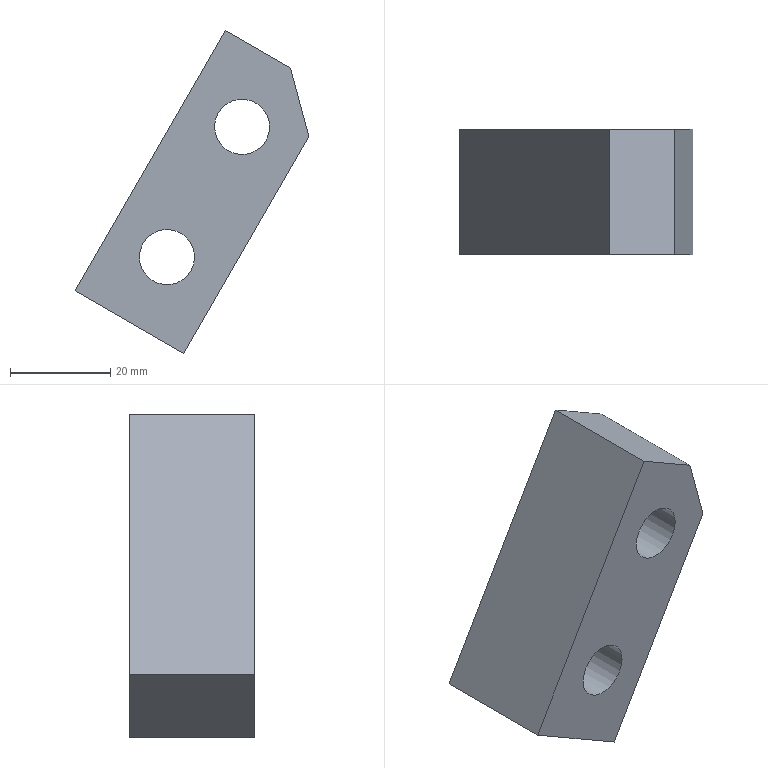Part | NX | features solid 2 | 1 solid | 13 faces | box 46.651 x 25 x 64.462 mm | volume 27133 mm3 | plane 9 | cylinder 4 | commonest cylinder face diameters 11 x2 17.5 x2
STEP:
#1=CARTESIAN_POINT('',(1078.617,295.,34.132));
#2=VERTEX_POINT('',#1);
#3=CARTESIAN_POINT('',(1091.607,295.,26.632));
#4=VERTEX_POINT('',#3);
#5=CARTESIAN_POINT('',(1087.726,295.,28.872));
#6=DIRECTION('',(0.866,0.,-0.5));
#7=VECTOR('',#6,1000.);
#8=LINE('',#5,#7);
#9=EDGE_CURVE('',#2,#4,#8,.T.);
#10=ORIENTED_EDGE('',*,*,#9,.F.);
#11=CARTESIAN_POINT('',(1078.617,270.,34.132));
#12=VERTEX_POINT('',#11);
#13=CARTESIAN_POINT('',(1078.617,270.,34.132));
#14=DIRECTION('',(0.,1.,0.));
#15=VECTOR('',#14,1000.);
#16=LINE('',#13,#15);
#17=EDGE_CURVE('',#12,#2,#16,.T.);
#18=ORIENTED_EDGE('',*,*,#17,.F.);
#19=CARTESIAN_POINT('',(1091.607,270.,26.632));
#20=VERTEX_POINT('',#19);
#21=CARTESIAN_POINT('',(1087.726,270.,28.872));
#22=DIRECTION('',(0.866,0.,-0.5));
#23=VECTOR('',#22,1000.);
#24=LINE('',#21,#23);
#25=EDGE_CURVE('',#12,#20,#24,.T.);
#26=ORIENTED_EDGE('',*,*,#25,.T.);
#27=CARTESIAN_POINT('',(1091.607,270.,26.632));
#28=DIRECTION('',(0.,1.,0.));
#29=VECTOR('',#28,1000.);
#30=LINE('',#27,#29);
#31=EDGE_CURVE('',#20,#4,#30,.T.);
#32=ORIENTED_EDGE('',*,*,#31,.T.);
#33=EDGE_LOOP('',(#10,#18,#26,#32));
#34=FACE_BOUND('',#33,.T.);
#35=CARTESIAN_POINT('',(1087.726,270.,28.872));
#36=DIRECTION('',(-0.5,0.,-0.866));
#37=DIRECTION('',(0.866,0.,-0.5));
#38=AXIS2_PLACEMENT_3D('',#35,#36,#37);
#39=PLANE('',#38);
#40=ADVANCED_FACE('',(#34),#39,.F.);
#41=CARTESIAN_POINT('',(1048.617,295.,-17.83));
#42=VERTEX_POINT('',#41);
#43=CARTESIAN_POINT('',(1075.343,295.,28.462));
#44=DIRECTION('',(-0.5,0.,-0.866));
#45=VECTOR('',#44,1000.);
#46=LINE('',#43,#45);
#47=EDGE_CURVE('',#42,#2,#46,.F.);
#48=ORIENTED_EDGE('',*,*,#47,.F.);
#49=CARTESIAN_POINT('',(1048.617,270.,-17.83));
#50=VERTEX_POINT('',#49);
#51=CARTESIAN_POINT('',(1048.617,270.,-17.83));
#52=DIRECTION('',(0.,1.,0.));
#53=VECTOR('',#52,1000.);
#54=LINE('',#51,#53);
#55=EDGE_CURVE('',#50,#42,#54,.T.);
#56=ORIENTED_EDGE('',*,*,#55,.F.);
#57=CARTESIAN_POINT('',(1075.343,270.,28.462));
#58=DIRECTION('',(-0.5,0.,-0.866));
#59=VECTOR('',#58,1000.);
#60=LINE('',#57,#59);
#61=EDGE_CURVE('',#50,#12,#60,.F.);
#62=ORIENTED_EDGE('',*,*,#61,.T.);
#63=ORIENTED_EDGE('',*,*,#17,.T.);
#64=EDGE_LOOP('',(#48,#56,#62,#63));
#65=FACE_BOUND('',#64,.T.);
#66=CARTESIAN_POINT('',(1075.343,270.,28.462));
#67=DIRECTION('',(0.866,0.,-0.5));
#68=DIRECTION('',(0.5,0.,0.866));
#69=AXIS2_PLACEMENT_3D('',#66,#67,#68);
#70=PLANE('',#69);
#71=ADVANCED_FACE('',(#65),#70,.F.);
#72=CARTESIAN_POINT('',(1070.268,295.,-30.33));
#73=VERTEX_POINT('',#72);
#74=CARTESIAN_POINT('',(1057.277,295.,-22.83));
#75=DIRECTION('',(0.866,0.,-0.5));
#76=VECTOR('',#75,1000.);
#77=LINE('',#74,#76);
#78=EDGE_CURVE('',#42,#73,#77,.T.);
#79=ORIENTED_EDGE('',*,*,#78,.T.);
#80=CARTESIAN_POINT('',(1070.268,270.,-30.33));
#81=VERTEX_POINT('',#80);
#82=CARTESIAN_POINT('',(1070.268,270.,-30.33));
#83=DIRECTION('',(0.,1.,0.));
#84=VECTOR('',#83,1000.);
#85=LINE('',#82,#84);
#86=EDGE_CURVE('',#81,#73,#85,.T.);
#87=ORIENTED_EDGE('',*,*,#86,.F.);
#88=CARTESIAN_POINT('',(1057.277,270.,-22.83));
#89=DIRECTION('',(0.866,0.,-0.5));
#90=VECTOR('',#89,1000.);
#91=LINE('',#88,#90);
#92=EDGE_CURVE('',#50,#81,#91,.T.);
#93=ORIENTED_EDGE('',*,*,#92,.F.);
#94=ORIENTED_EDGE('',*,*,#55,.T.);
#95=EDGE_LOOP('',(#79,#87,#93,#94));
#96=FACE_BOUND('',#95,.T.);
#97=CARTESIAN_POINT('',(1057.277,270.,-22.83));
#98=DIRECTION('',(-0.5,0.,-0.866));
#99=DIRECTION('',(0.866,0.,-0.5));
#100=AXIS2_PLACEMENT_3D('',#97,#98,#99);
#101=PLANE('',#100);
#102=ADVANCED_FACE('',(#96),#101,.T.);
#103=CARTESIAN_POINT('',(1095.268,295.,12.972));
#104=VERTEX_POINT('',#103);
#105=CARTESIAN_POINT('',(1061.518,295.,-45.485));
#106=DIRECTION('',(0.5,0.,0.866));
#107=VECTOR('',#106,1000.);
#108=LINE('',#105,#107);
#109=EDGE_CURVE('',#73,#104,#108,.T.);
#110=ORIENTED_EDGE('',*,*,#109,.T.);
#111=CARTESIAN_POINT('',(1095.268,270.,12.972));
#112=VERTEX_POINT('',#111);
#113=CARTESIAN_POINT('',(1095.268,270.,12.972));
#114=DIRECTION('',(0.,1.,0.));
#115=VECTOR('',#114,1000.);
#116=LINE('',#113,#115);
#117=EDGE_CURVE('',#112,#104,#116,.T.);
#118=ORIENTED_EDGE('',*,*,#117,.F.);
#119=CARTESIAN_POINT('',(1061.518,270.,-45.485));
#120=DIRECTION('',(0.5,0.,0.866));
#121=VECTOR('',#120,1000.);
#122=LINE('',#119,#121);
#123=EDGE_CURVE('',#81,#112,#122,.T.);
#124=ORIENTED_EDGE('',*,*,#123,.F.);
#125=ORIENTED_EDGE('',*,*,#86,.T.);
#126=EDGE_LOOP('',(#110,#118,#124,#125));
#127=FACE_BOUND('',#126,.T.);
#128=CARTESIAN_POINT('',(1061.518,270.,-45.485));
#129=DIRECTION('',(0.866,0.,-0.5));
#130=DIRECTION('',(0.5,0.,0.866));
#131=AXIS2_PLACEMENT_3D('',#128,#129,#130);
#132=PLANE('',#131);
#133=ADVANCED_FACE('',(#127),#132,.T.);
#134=CARTESIAN_POINT('',(1102.189,295.,-12.86));
#135=DIRECTION('',(-0.2588,0.,0.9659));
#136=VECTOR('',#135,1000.);
#137=LINE('',#134,#136);
#138=EDGE_CURVE('',#4,#104,#137,.F.);
#139=ORIENTED_EDGE('',*,*,#138,.F.);
#140=ORIENTED_EDGE('',*,*,#31,.F.);
#141=CARTESIAN_POINT('',(1102.189,270.,-12.86));
#142=DIRECTION('',(-0.2588,0.,0.9659));
#143=VECTOR('',#142,1000.);
#144=LINE('',#141,#143);
#145=EDGE_CURVE('',#20,#112,#144,.F.);
#146=ORIENTED_EDGE('',*,*,#145,.T.);
#147=ORIENTED_EDGE('',*,*,#117,.T.);
#148=EDGE_LOOP('',(#139,#140,#146,#147));
#149=FACE_BOUND('',#148,.T.);
#150=CARTESIAN_POINT('',(1102.189,270.,-12.86));
#151=DIRECTION('',(-0.9659,0.,-0.2588));
#152=DIRECTION('',(0.2588,0.,-0.9659));
#153=AXIS2_PLACEMENT_3D('',#150,#151,#152);
#154=PLANE('',#153);
#155=ADVANCED_FACE('',(#149),#154,.F.);
#156=CARTESIAN_POINT('',(1080.061,270.,20.06));
#157=VERTEX_POINT('',#156);
#158=CARTESIAN_POINT('',(1081.942,270.,14.891));
#159=DIRECTION('',(0.,-1.,0.));
#160=DIRECTION('',(-0.342,0.,0.9397));
#161=AXIS2_PLACEMENT_3D('',#158,#159,#160);
#162=CIRCLE('',#161,5.5);
#163=EDGE_CURVE('',#157,#157,#162,.T.);
#164=ORIENTED_EDGE('',*,*,#163,.F.);
#165=EDGE_LOOP('',(#164));
#166=FACE_BOUND('',#165,.T.);
#167=CARTESIAN_POINT('',(1065.061,270.,-5.921));
#168=VERTEX_POINT('',#167);
#169=CARTESIAN_POINT('',(1066.942,270.,-11.089));
#170=DIRECTION('',(0.,-1.,0.));
#171=DIRECTION('',(-0.342,0.,0.9397));
#172=AXIS2_PLACEMENT_3D('',#169,#170,#171);
#173=CIRCLE('',#172,5.5);
#174=EDGE_CURVE('',#168,#168,#173,.T.);
#175=ORIENTED_EDGE('',*,*,#174,.F.);
#176=EDGE_LOOP('',(#175));
#177=FACE_BOUND('',#176,.T.);
#178=ORIENTED_EDGE('',*,*,#25,.F.);
#179=ORIENTED_EDGE('',*,*,#61,.F.);
#180=ORIENTED_EDGE('',*,*,#92,.T.);
#181=ORIENTED_EDGE('',*,*,#123,.T.);
#182=ORIENTED_EDGE('',*,*,#145,.F.);
#183=EDGE_LOOP('',(#178,#179,#180,#181,#182));
#184=FACE_BOUND('',#183,.T.);
#185=CARTESIAN_POINT('',(1051.576,270.,-33.743));
#186=DIRECTION('',(0.,1.,0.));
#187=DIRECTION('',(0.342,0.,-0.9397));
#188=AXIS2_PLACEMENT_3D('',#185,#186,#187);
#189=PLANE('',#188);
#190=ADVANCED_FACE('',(#166,#177,#184),#189,.F.);
#191=CARTESIAN_POINT('',(1084.935,295.,6.669));
#192=VERTEX_POINT('',#191);
#193=CARTESIAN_POINT('',(1081.942,295.,14.891));
#194=DIRECTION('',(0.,1.,0.));
#195=DIRECTION('',(0.342,0.,-0.9397));
#196=AXIS2_PLACEMENT_3D('',#193,#194,#195);
#197=CIRCLE('',#196,8.75);
#198=EDGE_CURVE('',#192,#192,#197,.T.);
#199=ORIENTED_EDGE('',*,*,#198,.F.);
#200=EDGE_LOOP('',(#199));
#201=FACE_BOUND('',#200,.T.);
#202=CARTESIAN_POINT('',(1069.935,295.,-19.312));
#203=VERTEX_POINT('',#202);
#204=CARTESIAN_POINT('',(1066.942,295.,-11.089));
#205=DIRECTION('',(0.,1.,0.));
#206=DIRECTION('',(0.342,0.,-0.9397));
#207=AXIS2_PLACEMENT_3D('',#204,#205,#206);
#208=CIRCLE('',#207,8.75);
#209=EDGE_CURVE('',#203,#203,#208,.T.);
#210=ORIENTED_EDGE('',*,*,#209,.F.);
#211=EDGE_LOOP('',(#210));
#212=FACE_BOUND('',#211,.T.);
#213=ORIENTED_EDGE('',*,*,#9,.T.);
#214=ORIENTED_EDGE('',*,*,#138,.T.);
#215=ORIENTED_EDGE('',*,*,#109,.F.);
#216=ORIENTED_EDGE('',*,*,#78,.F.);
#217=ORIENTED_EDGE('',*,*,#47,.T.);
#218=EDGE_LOOP('',(#213,#214,#215,#216,#217));
#219=FACE_BOUND('',#218,.T.);
#220=CARTESIAN_POINT('',(1051.576,295.,-33.743));
#221=DIRECTION('',(0.,1.,0.));
#222=DIRECTION('',(0.342,0.,-0.9397));
#223=AXIS2_PLACEMENT_3D('',#220,#221,#222);
#224=PLANE('',#223);
#225=ADVANCED_FACE('',(#201,#212,#219),#224,.T.);
#226=CARTESIAN_POINT('',(1068.823,280.,-16.258));
#227=VERTEX_POINT('',#226);
#228=CARTESIAN_POINT('',(1066.942,280.,-11.089));
#229=DIRECTION('',(0.,1.,0.));
#230=DIRECTION('',(0.342,0.,-0.9397));
#231=AXIS2_PLACEMENT_3D('',#228,#229,#230);
#232=CIRCLE('',#231,5.5);
#233=EDGE_CURVE('',#227,#227,#232,.T.);
#234=ORIENTED_EDGE('',*,*,#233,.T.);
#235=EDGE_LOOP('',(#234));
#236=FACE_BOUND('',#235,.T.);
#237=ORIENTED_EDGE('',*,*,#174,.T.);
#238=EDGE_LOOP('',(#237));
#239=FACE_BOUND('',#238,.T.);
#240=CARTESIAN_POINT('',(1066.942,245.,-11.089));
#241=DIRECTION('',(0.,-1.,0.));
#242=DIRECTION('',(0.342,0.,-0.9397));
#243=AXIS2_PLACEMENT_3D('',#240,#241,#242);
#244=CYLINDRICAL_SURFACE('',#243,5.5);
#245=ADVANCED_FACE('',(#236,#239),#244,.F.);
#246=ORIENTED_EDGE('',*,*,#233,.F.);
#247=EDGE_LOOP('',(#246));
#248=FACE_BOUND('',#247,.T.);
#249=CARTESIAN_POINT('',(1069.935,280.,-19.312));
#250=VERTEX_POINT('',#249);
#251=CARTESIAN_POINT('',(1066.942,280.,-11.089));
#252=DIRECTION('',(0.,1.,0.));
#253=DIRECTION('',(0.342,0.,-0.9397));
#254=AXIS2_PLACEMENT_3D('',#251,#252,#253);
#255=CIRCLE('',#254,8.75);
#256=EDGE_CURVE('',#250,#250,#255,.T.);
#257=ORIENTED_EDGE('',*,*,#256,.T.);
#258=EDGE_LOOP('',(#257));
#259=FACE_BOUND('',#258,.T.);
#260=CARTESIAN_POINT('',(1066.942,280.,-11.089));
#261=DIRECTION('',(0.,-1.,0.));
#262=DIRECTION('',(0.342,0.,-0.9397));
#263=AXIS2_PLACEMENT_3D('',#260,#261,#262);
#264=PLANE('',#263);
#265=ADVANCED_FACE('',(#248,#259),#264,.F.);
#266=ORIENTED_EDGE('',*,*,#256,.F.);
#267=EDGE_LOOP('',(#266));
#268=FACE_BOUND('',#267,.T.);
#269=ORIENTED_EDGE('',*,*,#209,.T.);
#270=EDGE_LOOP('',(#269));
#271=FACE_BOUND('',#270,.T.);
#272=CARTESIAN_POINT('',(1066.942,295.,-11.089));
#273=DIRECTION('',(0.,-1.,0.));
#274=DIRECTION('',(0.342,0.,-0.9397));
#275=AXIS2_PLACEMENT_3D('',#272,#273,#274);
#276=CYLINDRICAL_SURFACE('',#275,8.75);
#277=ADVANCED_FACE('',(#268,#271),#276,.F.);
#278=CARTESIAN_POINT('',(1083.823,280.,9.723));
#279=VERTEX_POINT('',#278);
#280=CARTESIAN_POINT('',(1081.942,280.,14.891));
#281=DIRECTION('',(0.,1.,0.));
#282=DIRECTION('',(0.342,0.,-0.9397));
#283=AXIS2_PLACEMENT_3D('',#280,#281,#282);
#284=CIRCLE('',#283,5.5);
#285=EDGE_CURVE('',#279,#279,#284,.T.);
#286=ORIENTED_EDGE('',*,*,#285,.T.);
#287=EDGE_LOOP('',(#286));
#288=FACE_BOUND('',#287,.T.);
#289=ORIENTED_EDGE('',*,*,#163,.T.);
#290=EDGE_LOOP('',(#289));
#291=FACE_BOUND('',#290,.T.);
#292=CARTESIAN_POINT('',(1081.942,245.,14.891));
#293=DIRECTION('',(0.,-1.,0.));
#294=DIRECTION('',(0.342,0.,-0.9397));
#295=AXIS2_PLACEMENT_3D('',#292,#293,#294);
#296=CYLINDRICAL_SURFACE('',#295,5.5);
#297=ADVANCED_FACE('',(#288,#291),#296,.F.);
#298=ORIENTED_EDGE('',*,*,#285,.F.);
#299=EDGE_LOOP('',(#298));
#300=FACE_BOUND('',#299,.T.);
#301=CARTESIAN_POINT('',(1084.935,280.,6.669));
#302=VERTEX_POINT('',#301);
#303=CARTESIAN_POINT('',(1081.942,280.,14.891));
#304=DIRECTION('',(0.,1.,0.));
#305=DIRECTION('',(0.342,0.,-0.9397));
#306=AXIS2_PLACEMENT_3D('',#303,#304,#305);
#307=CIRCLE('',#306,8.75);
#308=EDGE_CURVE('',#302,#302,#307,.T.);
#309=ORIENTED_EDGE('',*,*,#308,.T.);
#310=EDGE_LOOP('',(#309));
#311=FACE_BOUND('',#310,.T.);
#312=CARTESIAN_POINT('',(1081.942,280.,14.891));
#313=DIRECTION('',(0.,-1.,0.));
#314=DIRECTION('',(0.342,0.,-0.9397));
#315=AXIS2_PLACEMENT_3D('',#312,#313,#314);
#316=PLANE('',#315);
#317=ADVANCED_FACE('',(#300,#311),#316,.F.);
#318=ORIENTED_EDGE('',*,*,#308,.F.);
#319=EDGE_LOOP('',(#318));
#320=FACE_BOUND('',#319,.T.);
#321=ORIENTED_EDGE('',*,*,#198,.T.);
#322=EDGE_LOOP('',(#321));
#323=FACE_BOUND('',#322,.T.);
#324=CARTESIAN_POINT('',(1081.942,295.,14.891));
#325=DIRECTION('',(0.,-1.,0.));
#326=DIRECTION('',(0.342,0.,-0.9397));
#327=AXIS2_PLACEMENT_3D('',#324,#325,#326);
#328=CYLINDRICAL_SURFACE('',#327,8.75);
#329=ADVANCED_FACE('',(#320,#323),#328,.F.);
#330=CLOSED_SHELL('',(#40,#71,#102,#133,#155,#190,#225,#245,#265,#277,#297,#317,#329));
#331=MANIFOLD_SOLID_BREP('',#330);
#332=(LENGTH_UNIT()NAMED_UNIT(*)SI_UNIT(.MILLI.,.METRE.));
#333=UNCERTAINTY_MEASURE_WITH_UNIT(LENGTH_MEASURE(0.00001),#332,'','');
#334=(NAMED_UNIT(*)PLANE_ANGLE_UNIT()SI_UNIT($,.RADIAN.));
#335=(NAMED_UNIT(*)SI_UNIT($,.STERADIAN.)SOLID_ANGLE_UNIT());
#336=(GEOMETRIC_REPRESENTATION_CONTEXT(3)GLOBAL_UNCERTAINTY_ASSIGNED_CONTEXT((#333))GLOBAL_UNIT_ASSIGNED_CONTEXT((#332,#334,#335))REPRESENTATION_CONTEXT('',''));
#337=ADVANCED_BREP_SHAPE_REPRESENTATION('',(#331),#336);